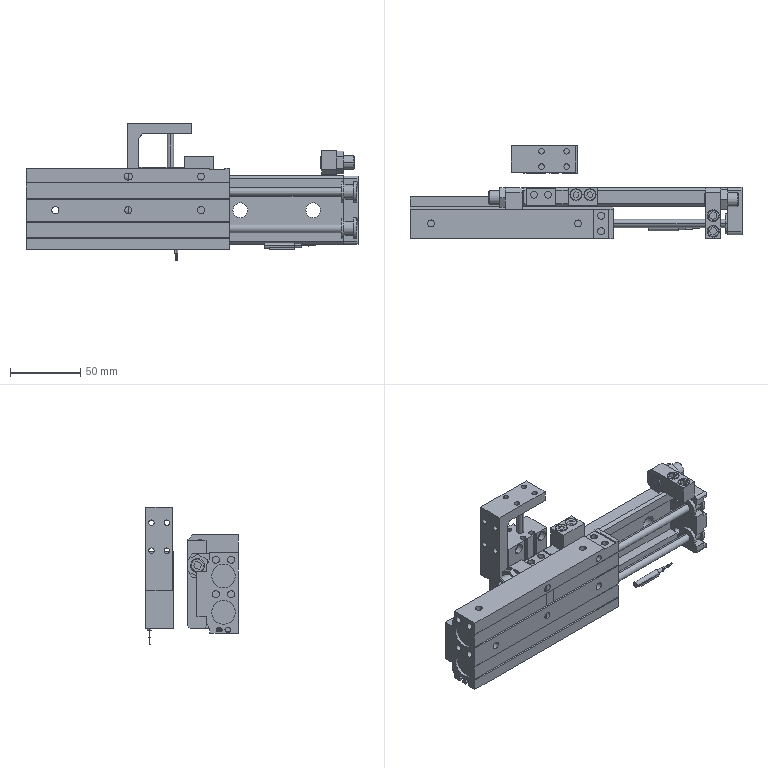Part | NX | 13 solids | 725 faces | box 237 x 67 x 98 mm | volume 330145 mm3 | plane 408 | cylinder 293 | cone 24 | commonest cylinder face diameters 5 x74 4 x44 0.5 x16 1 x16 8.5 x16 10 x15